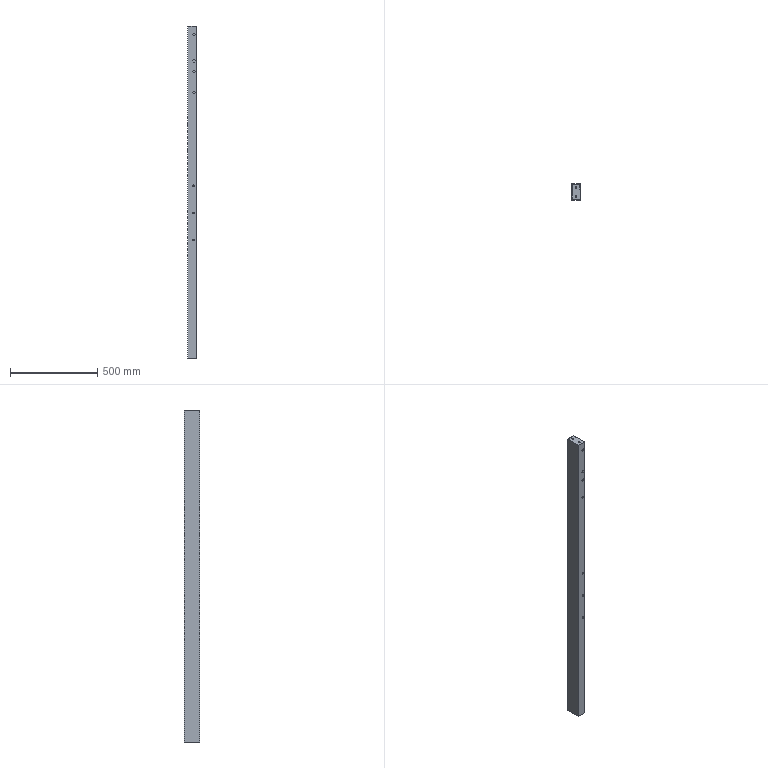Part | SolidWorks | features BaseBody 1 | 1 solid | 51 faces | box 50 x 90 x 1900 mm | volume 1026143 mm3 | plane 37 | cylinder 14 | commonest cylinder face diameters 11 x8 10.6 x6